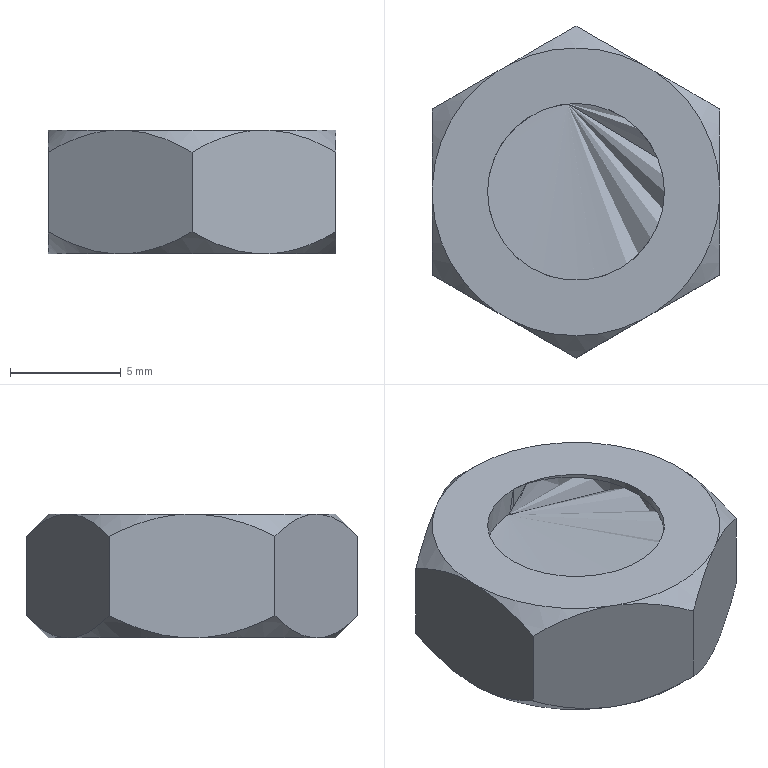Part | SolidWorks | features BaseBody 1 | 1 solid | 42 faces | box 13 x 15.011 x 5.606 mm | volume 605.812 mm3 | cone 12 | spline 12 | cylinder 10 | plane 8 | commonest cylinder face diameters 8 x10